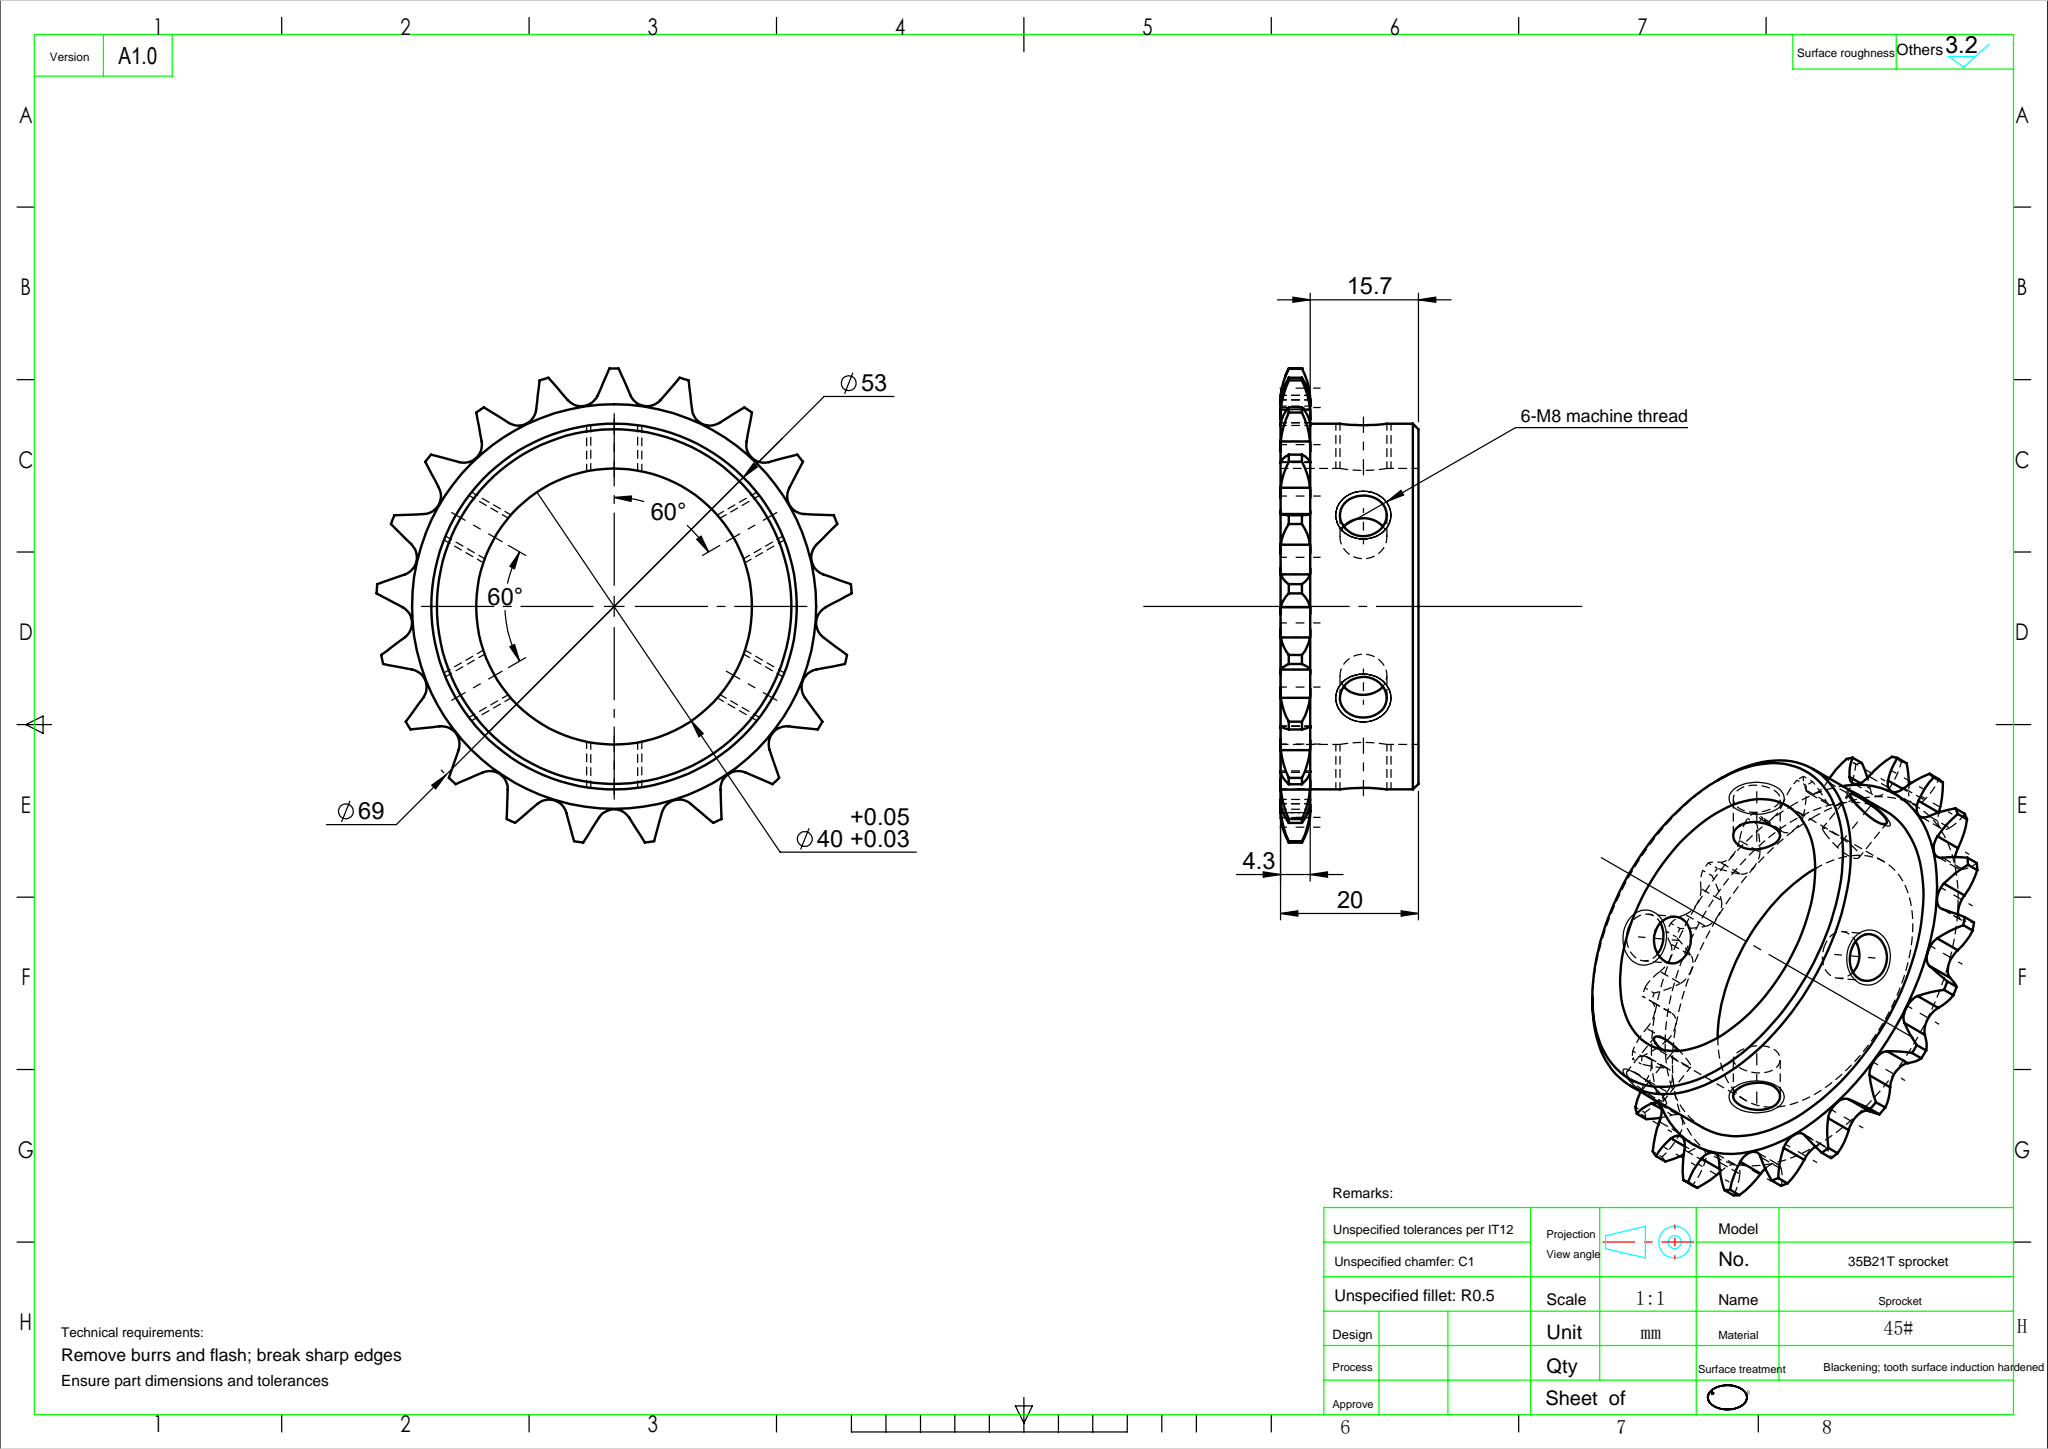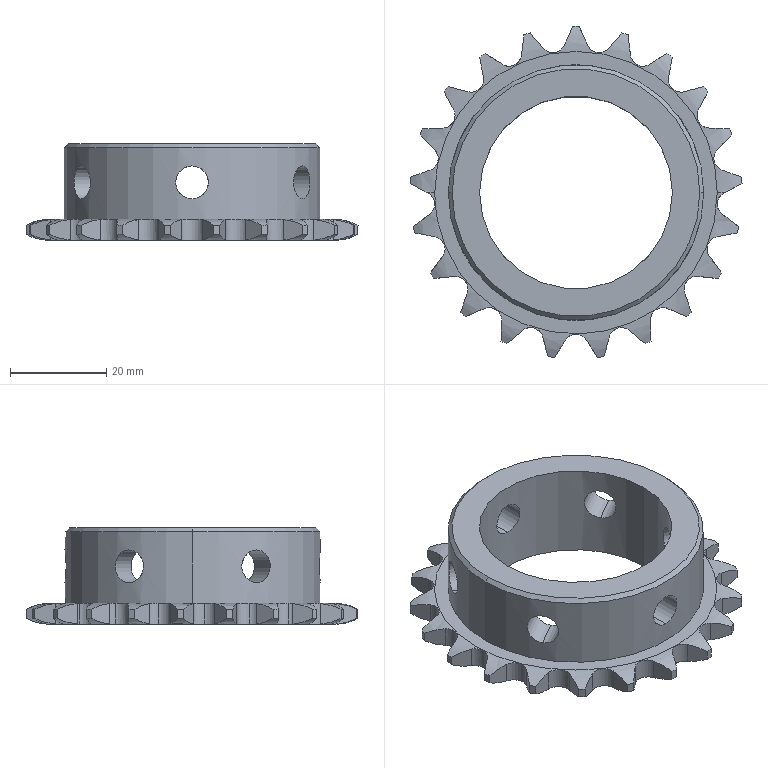Part | SolidWorks | features DelFace 2, ICE 2, BaseBody 1, CirPattern 1 | 1 solid | 116 faces | box 69 x 68.708 x 20.007 mm | volume 21255 mm3 | cylinder 65 | plane 45 | spline 4 | cone 2 | commonest cylinder face diameters 5.2 x28 69 x21 6.8 x12 40 x2 53 x2